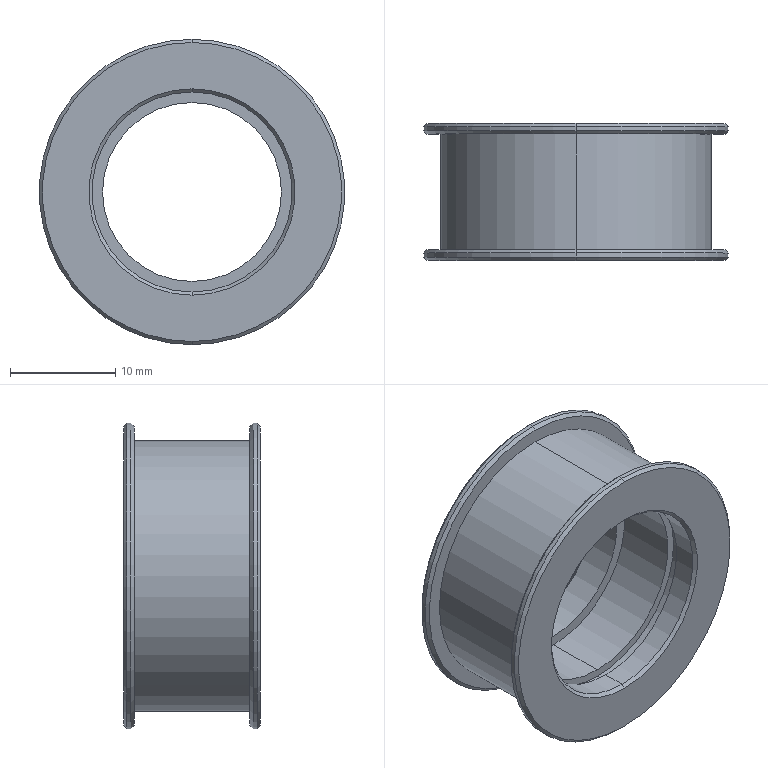Part | STEP file | 1 solid | 33 faces | box 29 x 13 x 29 mm | volume 3455 mm3 | cylinder 14 | cone 12 | plane 7 | commonest cylinder face diameters 19 x4 29 x4 17 x2 20.5 x2 25.68 x2